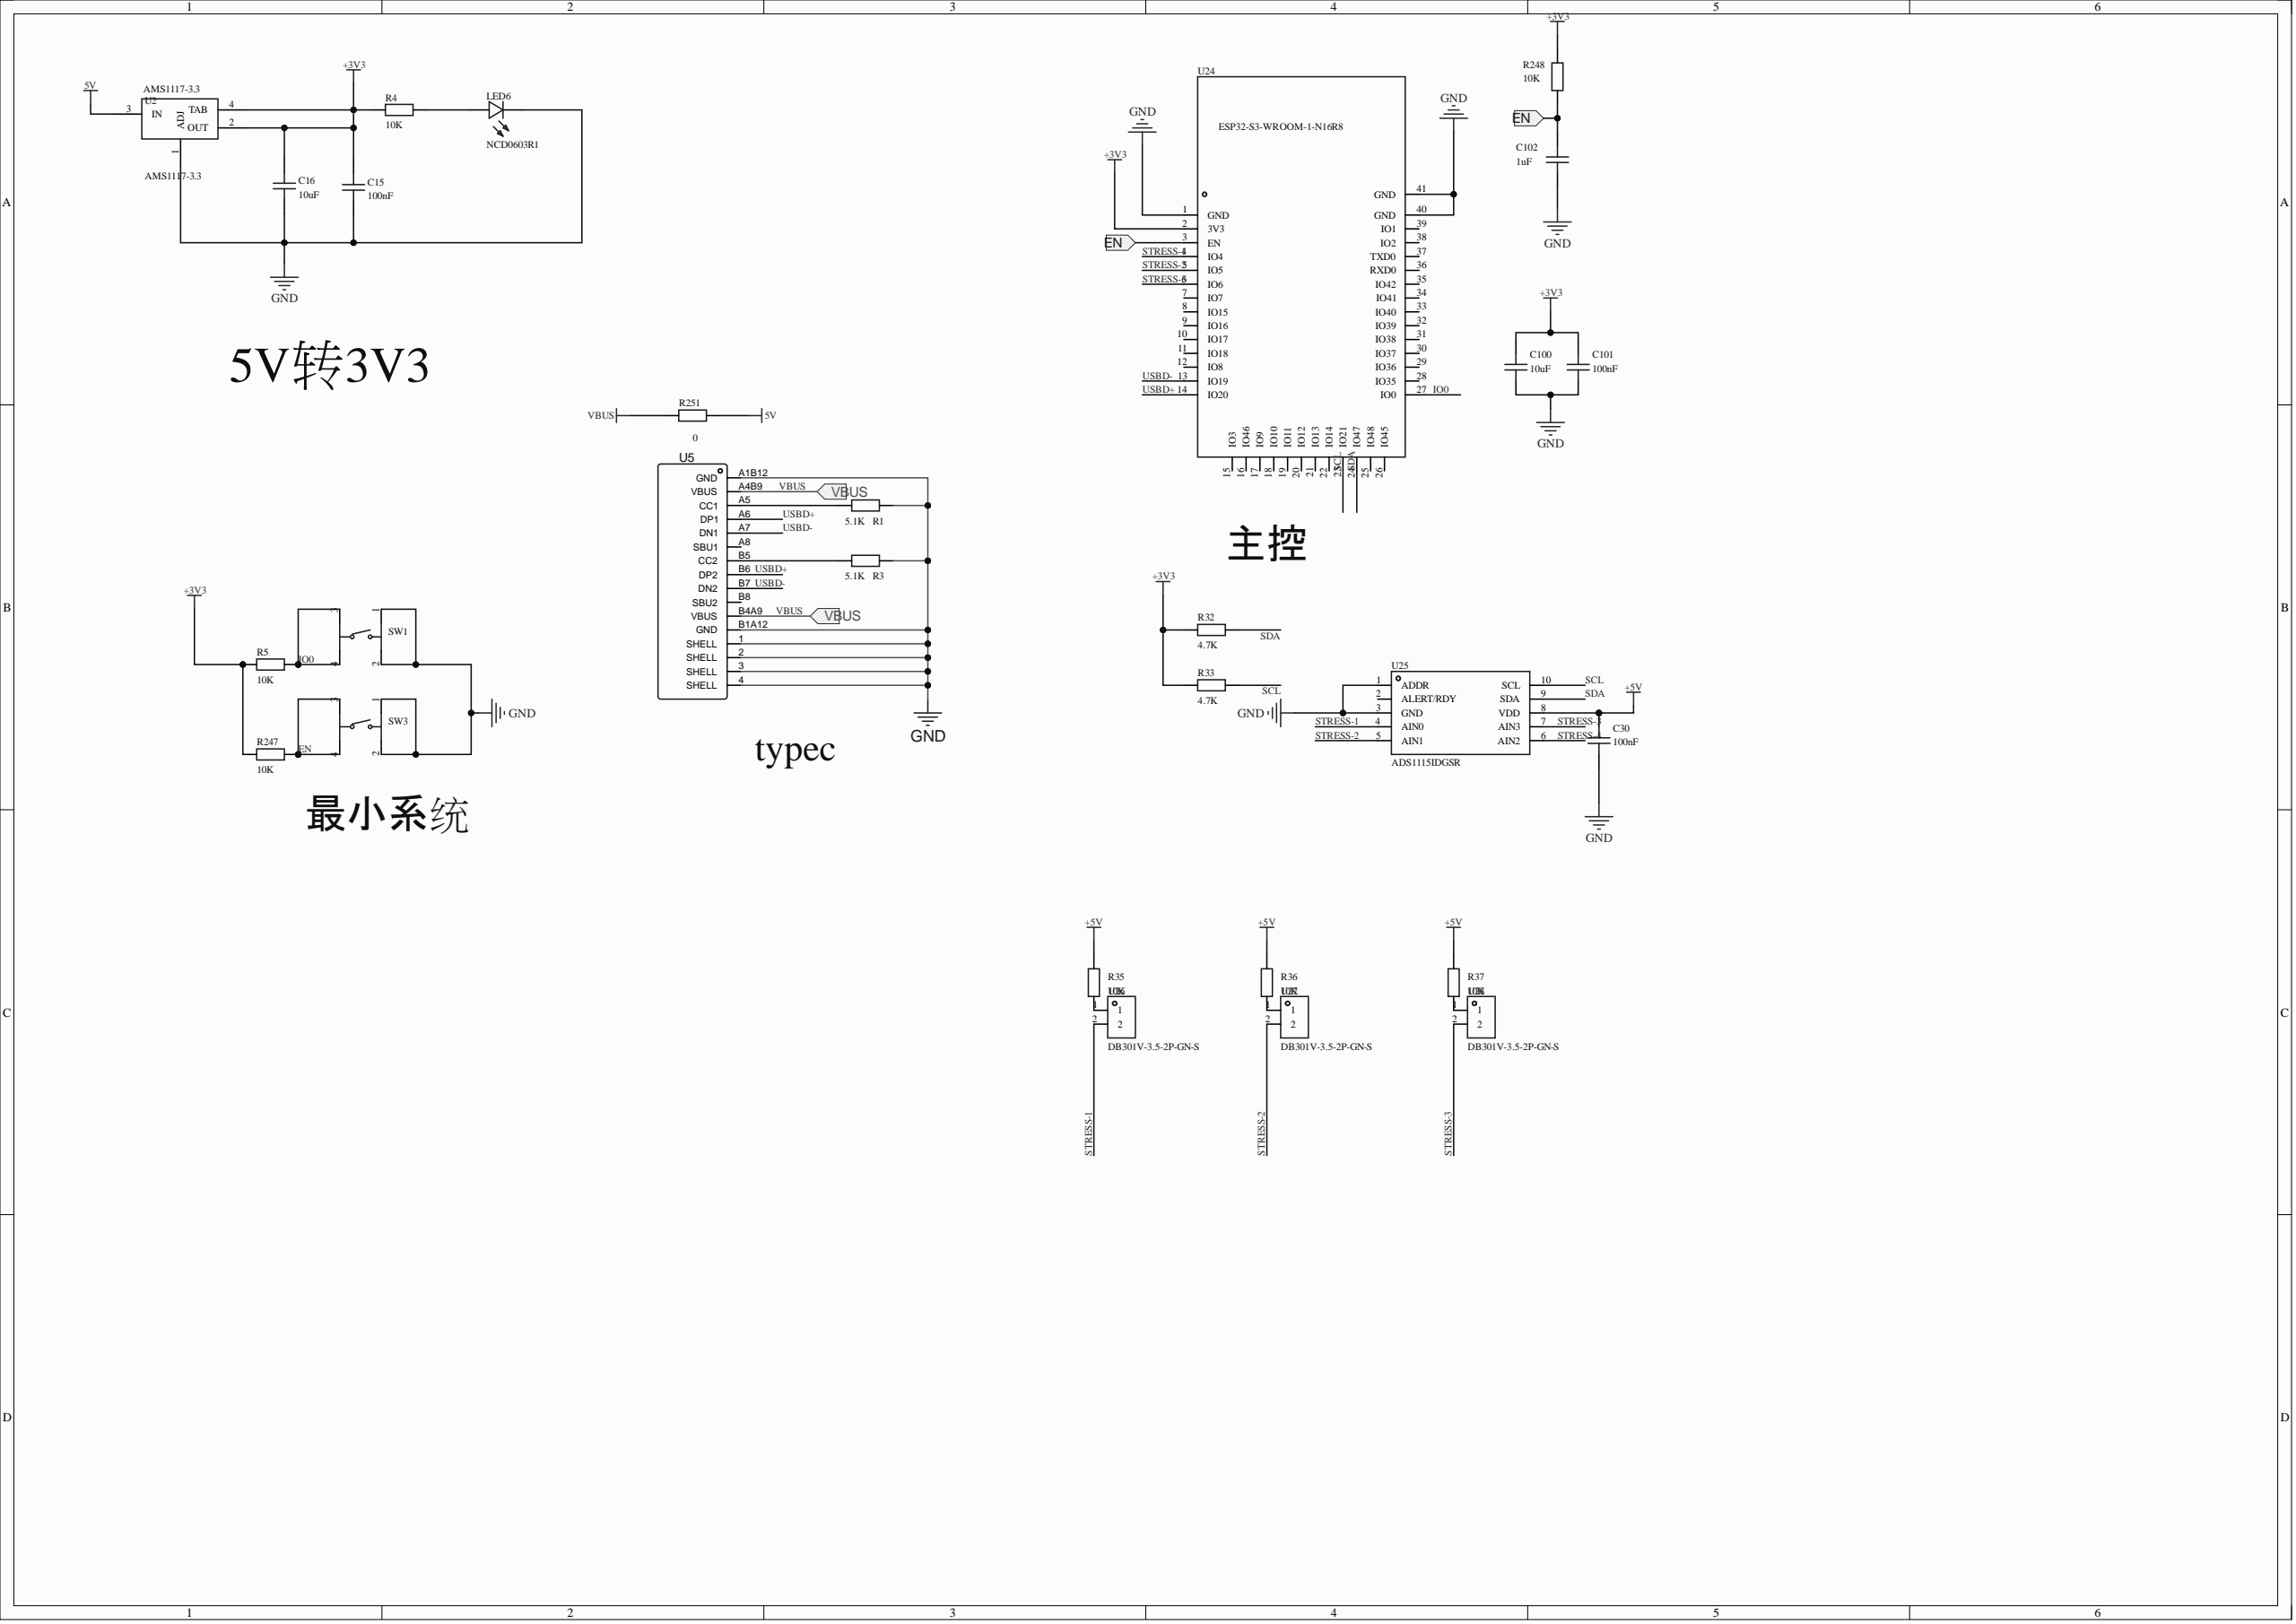Circuit board | Altium Designer | 28 parts | 21 nets
Bill of materials:
Comment,Description,Designator,Footprint,LibRef,Quantity
"100nF","","C15, C101","C0402","CAP_0402, 0603F104Z500CT_C83060","2"
"10uF","","C16, C100","C0402","CAP_0402, CL10A105KB8NNNC","2"
"100nF","容值:100nF;精度:-20%~+80%;额定电压:50V;材质(温度系数):Y5V;","C30","C0603","0603F104Z500CT_C83060","1"
"1uF","","C102","C0402","CAP_0603","1"
"NCD0603R1","灯头类型:-;发光颜色:红色;正向电压(VF):1.6V~2.6V;功率:65mW;正向电流:20mA;主波长:615nm~630nm;二极管配置:独立二极管;透镜颜色:无色透明透镜;色温:-;发光强度:80mcd~220mcd;发光角度:130°;载带方式:-;工作温度:-30℃~+85℃;","LED6","LED0603-RD_RED","NCD0603R1_C84263","1"
"5.1K","","R1, R3","r0402","Res_0603","2"
"10K","","R4, R5, R247","r0402","Res_0603","3"
"Res_0603","","R32, R33, R35, R36, R37","R0603","Res_0603","5"
"","","R248","r0402","Res_0603","1"
"0","","R251","r0402","Res_0603","1"
"TS-1089S-02526","电路结构:单刀单掷;按钮形状:椭圆形按钮;安装方式:立贴;开关长度:4.2mm;开关宽度:3.25mm;开关高度:2.5mm;触点电流:50mA;额定电压(DC):12V;带灯:-;机械寿命:-;","SW1, SW3","SW-SMD_4P-L4.2-W3.3-P2.15-LS5.1","TS-1089S-02526","2"
"AMS1117-3.3","","U2","sot-223(gd32)","AMS1117-3.3","1"
"TYPE-C16P","UART","U5","USB-C-SMD_TYPE-C16PIN-SHOUHAN","TYPE-C16P","1"
"ESP32-S3-WROOM-1-N16R8","","U24","WIRELM-SMD_ESP32-S3-WROOM-1","ESP32-S3-WROOM-1-N16R8","1"
"ADS1115IDGSR","接口:I2C;电源电压:2V~5.5V;采样率:860Hz;分辨率:16位;","U25","MSOP-10_L3.0-W3.0-P0.50-LS5.0-BL","ADS1115IDGSR","1"
"DB301V-3.5-2P-GN-S","结构:1x2P;间距:3.5mm;颜色:绿色;安装方式:直插;额定电流:10A;额定电压:130V;排数:1;线规 - AWG:18~24;线规 - 平方毫米:0.5~1;每排PIN数:2;工作温度范围:-40℃~+105℃;","U26, U27, U28","CONN-TH_DB301V-3.5-2P-GN","DB301V-3.5-2P-GN-S","3"
Netlist (Protel format):
[
C15
C0402
100nF



]
[
C16
C0402
10uF



]
[
C30
C0603
100nF



]
[
C100
C0402
10uF



]
[
C101
C0402
100nF



]
[
C102
C0402
1uF



]
[
LED6
LED0603-RD_RED
NCD0603R1



]
[
R1
r0402
5.1K



]
[
R3
r0402
5.1K



]
[
R4
r0402
10K



]
[
R5
r0402
10K



]
[
R32
R0603
Res_0603



]
[
R33
R0603
Res_0603



]
[
R35
R0603
Res_0603



]
[
R36
R0603
Res_0603



]
[
R37
R0603
Res_0603



]
[
R247
r0402
10K



]
[
R248
r0402




]
[
R251
r0402
0



]
[
SW1
SW-SMD_4P-L4.2-W3.3-P2.15-LS5.1
TS-1089S-02526



]
[
SW3
SW-SMD_4P-L4.2-W3.3-P2.15-LS5.1
TS-1089S-02526



]
[
U2
sot-223(gd32)
AMS1117-3.3



]
[
U5
USB-C-SMD_TYPE-C16PIN-SHOUHAN
TYPE-C16P



]
[
U24
WIRELM-SMD_ESP32-S3-WROOM-1
ESP32-S3-WROOM-1-N16R8



]
[
U25
MSOP-10_L3.0-W3.0-P0.50-LS5.0-BL
ADS1115IDGSR



]
[
U26
CONN-TH_DB301V-3.5-2P-GN
DB301V-3.5-2P-GN-S



]
[
U27
CONN-TH_DB301V-3.5-2P-GN
DB301V-3.5-2P-GN-S



]
[
U28
CONN-TH_DB301V-3.5-2P-GN
DB301V-3.5-2P-GN-S



]
(
VBUS
R251-1
U5-A4B9
U5-B4A9
)
(
USBD-
U5-A7
U5-B7
U24-13
)
(
USBD+
U5-A6
U5-B6
U24-14
)
(
STRESS-3
U24-6
U25-7
U28-2
)
(
STRESS-2
U24-5
U25-5
U27-2
)
(
STRESS-1
U24-4
U25-4
U26-2
)
(
SDA
R32-1
U24-24
U25-9
)
(
SCL
R33-1
U24-23
U25-10
)
(
NetR37_1
R37-1
U28-1
)
(
NetR36_1
R36-1
U27-1
)
(
NetR35_1
R35-1
U26-1
)
(
NetR3_1
R3-1
U5-B5
)
(
NetR1_1
R1-1
U5-A5
)
(
NetLED6_2
LED6-2
R4-2
)
(
NetC102_2
C102-2
R248-1
U24-3
)
(
IO0
R5-2
SW1-3
SW1-4
U24-27
)
(
GND
C15-1
C16-1
C30-1
C100-1
C101-1
C102-1
LED6-1
R1-2
R3-2
SW1-1
SW1-2
SW3-1
SW3-2
U2-1
U5-1
U5-2
U5-3
U5-4
U5-A1B12
U5-B1A12
U24-1
U24-40
U24-41
U25-1
U25-3
)
(
EN
R247-2
SW3-3
SW3-4
)
(
+5V
C30-2
R35-2
R36-2
R37-2
U25-8
)
(
+3V3
C15-2
C16-2
C100-2
C101-2
R4-1
R5-1
R32-2
R33-2
R247-1
R248-2
U2-2
U2-4
U24-2
)
(
5V
R251-2
U2-3
)